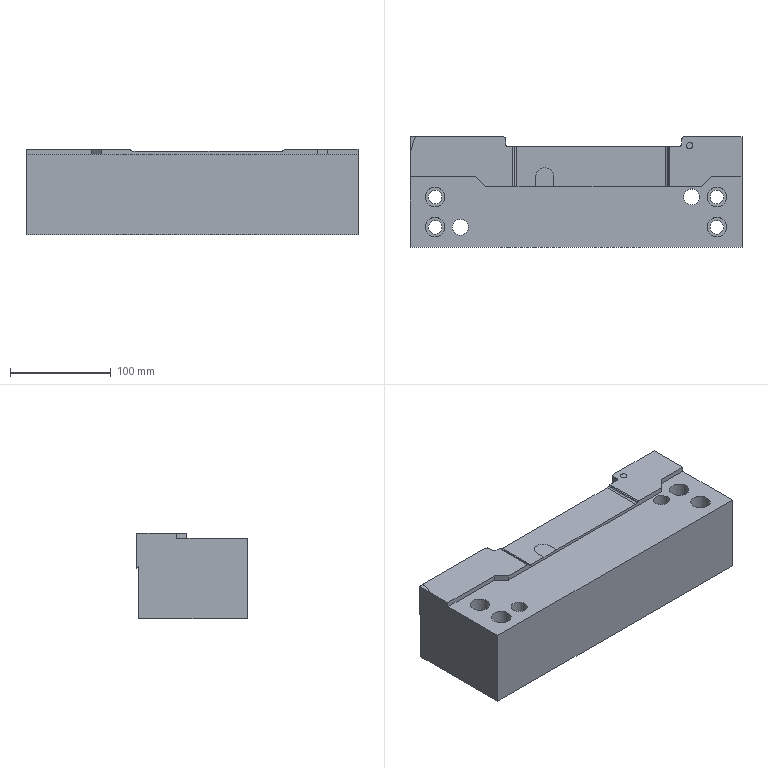Part | NX | features solid 2 | 1 solid | 47 faces | box 330 x 110 x 85 mm | volume 2709450 mm3 | spline 23 | plane 14 | cylinder 10 | commonest cylinder face diameters 13.5 x4 19.5 x4 16 x2